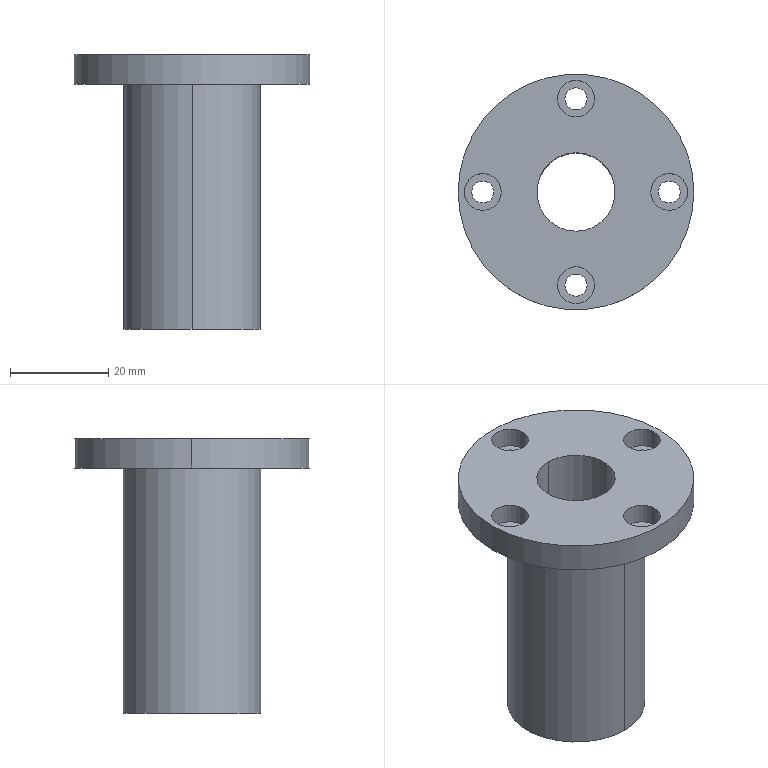Part | STEP file | Linear bearing LHFRD 16 | 1 solid | 29 faces | box 48 x 48 x 56 mm | volume 29540 mm3 | cylinder 22 | plane 7 | commonest cylinder face diameters 4.5 x8 7.5 x8 16 x2 28 x2 48 x2